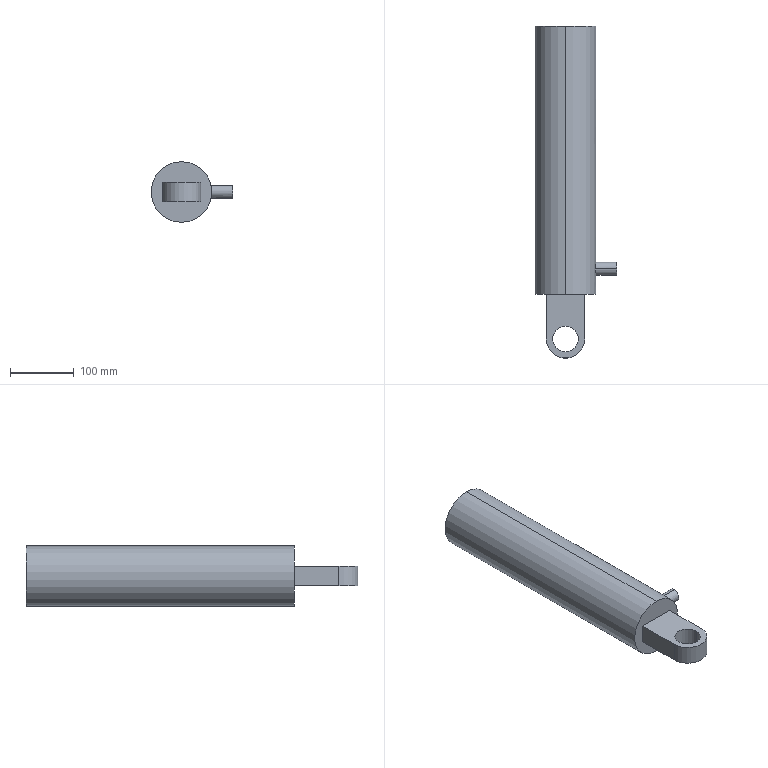Part | STEP file | Hydraulic cylinder body SLDPRT | 1 solid | 20 faces | box 127.5 x 520 x 95 mm | volume 2648079 mm3 | cylinder 12 | plane 8 | commonest cylinder face diameters 40 x4 95 x3 14 x2 20 x2 60 x1
STEP:
#1=CARTESIAN_POINT('',(80.,110.,22.));
#2=VERTEX_POINT('',#1);
#3=CARTESIAN_POINT('',(80.,110.,8.));
#4=VERTEX_POINT('',#3);
#5=CARTESIAN_POINT('',(80.,110.,15.));
#6=DIRECTION('',(1.,0.,0.));
#7=DIRECTION('',(0.,0.,-1.));
#8=AXIS2_PLACEMENT_3D('',#5,#6,#7);
#9=CIRCLE('',#8,7.);
#10=EDGE_CURVE('',#2,#4,#9,.T.);
#11=ORIENTED_EDGE('',*,*,#10,.T.);
#12=CARTESIAN_POINT('',(46.981,110.,8.));
#13=VERTEX_POINT('',#12);
#14=CARTESIAN_POINT('',(80.,110.,8.));
#15=DIRECTION('',(-1.,0.,0.));
#16=VECTOR('',#15,1000.);
#17=LINE('',#14,#16);
#18=EDGE_CURVE('',#4,#13,#17,.T.);
#19=ORIENTED_EDGE('',*,*,#18,.T.);
#20=CARTESIAN_POINT('',(46.981,110.,22.));
#21=VERTEX_POINT('',#20);
#22=CARTESIAN_POINT('',(46.981,110.,22.));
#23=CARTESIAN_POINT('',(46.981,109.537,22.));
#24=CARTESIAN_POINT('',(46.988,109.081,21.954));
#25=CARTESIAN_POINT('',(47.008,108.41,21.821));
#26=CARTESIAN_POINT('',(47.016,108.188,21.765));
#27=CARTESIAN_POINT('',(47.035,107.748,21.632));
#28=CARTESIAN_POINT('',(47.046,107.529,21.553));
#29=CARTESIAN_POINT('',(47.082,106.893,21.29));
#30=CARTESIAN_POINT('',(47.111,106.492,21.075));
#31=CARTESIAN_POINT('',(47.173,105.731,20.567));
#32=CARTESIAN_POINT('',(47.208,105.372,20.271));
#33=CARTESIAN_POINT('',(47.275,104.727,19.626));
#34=CARTESIAN_POINT('',(47.309,104.437,19.274));
#35=CARTESIAN_POINT('',(47.356,104.054,18.7));
#36=CARTESIAN_POINT('',(47.371,103.935,18.502));
#37=CARTESIAN_POINT('',(47.399,103.719,18.098));
#38=CARTESIAN_POINT('',(47.425,103.524,17.686));
#39=CARTESIAN_POINT('',(47.447,103.37,17.256));
#40=CARTESIAN_POINT('',(47.466,103.236,16.817));
#41=CARTESIAN_POINT('',(47.474,103.18,16.593));
#42=CARTESIAN_POINT('',(47.493,103.045,15.915));
#43=CARTESIAN_POINT('',(47.5,103.,15.46));
#44=CARTESIAN_POINT('',(47.5,103.,14.545));
#45=CARTESIAN_POINT('',(47.493,103.046,14.081));
#46=CARTESIAN_POINT('',(47.467,103.225,13.183));
#47=CARTESIAN_POINT('',(47.448,103.357,12.746));
#48=CARTESIAN_POINT('',(47.412,103.62,12.11));
#49=CARTESIAN_POINT('',(47.399,103.72,11.9));
#50=CARTESIAN_POINT('',(47.371,103.936,11.495));
#51=CARTESIAN_POINT('',(47.356,104.054,11.299));
#52=CARTESIAN_POINT('',(47.309,104.434,10.731));
#53=CARTESIAN_POINT('',(47.276,104.724,10.377));
#54=CARTESIAN_POINT('',(47.207,105.376,9.724));
#55=CARTESIAN_POINT('',(47.174,105.729,9.435));
#56=CARTESIAN_POINT('',(47.127,106.297,9.055));
#57=CARTESIAN_POINT('',(47.112,106.493,8.937));
#58=CARTESIAN_POINT('',(47.083,106.899,8.72));
#59=CARTESIAN_POINT('',(47.07,107.108,8.621));
#60=CARTESIAN_POINT('',(47.034,107.744,8.358));
#61=CARTESIAN_POINT('',(47.014,108.18,8.225));
#62=CARTESIAN_POINT('',(46.988,109.078,8.046));
#63=CARTESIAN_POINT('',(46.981,109.543,8.));
#64=CARTESIAN_POINT('',(46.981,110.,8.));
#65=B_SPLINE_CURVE_WITH_KNOTS('',3,(#22,#23,#24,#25,#26,#27,#28,#29,#30,#31,#32,#33,#34,#35,#36,#37,#38,#39,#40,#41,#42,#43,#44,#45,#46,#47,#48,#49,#50,#51,#52,#53,#54,#55,#56,#57,#58,#59,#60,#61,#62,#63,#64),.UNSPECIFIED.,.F.,.F.,(4,2,2,2,2,2,2,2,1,2,2,2,2,2,2,2,2,2,2,2,2,4),(0.,0.00137,0.002055,0.002739,0.004109,0.005479,0.006848,0.007533,0.008218,0.008903,0.009588,0.01096,0.01233,0.0137,0.01438,0.01507,0.01644,0.01781,0.01849,0.01918,0.02055,0.02192),.UNSPECIFIED.);
#66=EDGE_CURVE('',#21,#13,#65,.T.);
#67=ORIENTED_EDGE('',*,*,#66,.F.);
#68=CARTESIAN_POINT('',(80.,110.,22.));
#69=DIRECTION('',(-1.,0.,0.));
#70=VECTOR('',#69,1000.);
#71=LINE('',#68,#70);
#72=EDGE_CURVE('',#2,#21,#71,.T.);
#73=ORIENTED_EDGE('',*,*,#72,.F.);
#74=EDGE_LOOP('',(#11,#19,#67,#73));
#75=FACE_OUTER_BOUND('',#74,.T.);
#76=CARTESIAN_POINT('',(80.,110.,15.));
#77=DIRECTION('',(-1.,0.,0.));
#78=DIRECTION('',(0.,0.,1.));
#79=AXIS2_PLACEMENT_3D('',#76,#77,#78);
#80=CYLINDRICAL_SURFACE('',#79,7.);
#81=ADVANCED_FACE('',(#75),#80,.F.);
#82=CARTESIAN_POINT('',(80.,110.,5.));
#83=VERTEX_POINT('',#82);
#84=CARTESIAN_POINT('',(80.,110.,25.));
#85=VERTEX_POINT('',#84);
#86=CARTESIAN_POINT('',(80.,110.,15.));
#87=DIRECTION('',(1.,0.,0.));
#88=DIRECTION('',(0.,0.,-1.));
#89=AXIS2_PLACEMENT_3D('',#86,#87,#88);
#90=CIRCLE('',#89,10.);
#91=EDGE_CURVE('',#83,#85,#90,.T.);
#92=ORIENTED_EDGE('',*,*,#91,.F.);
#93=CARTESIAN_POINT('',(46.435,110.,5.));
#94=VERTEX_POINT('',#93);
#95=CARTESIAN_POINT('',(80.,110.,5.));
#96=DIRECTION('',(-1.,0.,0.));
#97=VECTOR('',#96,1000.);
#98=LINE('',#95,#97);
#99=EDGE_CURVE('',#83,#94,#98,.T.);
#100=ORIENTED_EDGE('',*,*,#99,.T.);
#101=CARTESIAN_POINT('',(46.435,110.,25.));
#102=VERTEX_POINT('',#101);
#103=CARTESIAN_POINT('',(46.435,110.,5.));
#104=CARTESIAN_POINT('',(46.435,110.653,5.));
#105=CARTESIAN_POINT('',(46.449,111.304,5.063));
#106=CARTESIAN_POINT('',(46.504,112.6,5.321));
#107=CARTESIAN_POINT('',(46.544,113.228,5.513));
#108=CARTESIAN_POINT('',(46.618,114.131,5.887));
#109=CARTESIAN_POINT('',(46.645,114.426,6.027));
#110=CARTESIAN_POINT('',(46.703,115.004,6.336));
#111=CARTESIAN_POINT('',(46.735,115.288,6.506));
#112=CARTESIAN_POINT('',(46.832,116.104,7.052));
#113=CARTESIAN_POINT('',(46.901,116.606,7.464));
#114=CARTESIAN_POINT('',(47.005,117.298,8.155));
#115=CARTESIAN_POINT('',(47.04,117.519,8.399));
#116=CARTESIAN_POINT('',(47.108,117.936,8.906));
#117=CARTESIAN_POINT('',(47.142,118.13,9.169));
#118=CARTESIAN_POINT('',(47.237,118.673,9.98));
#119=CARTESIAN_POINT('',(47.295,118.981,10.554));
#120=CARTESIAN_POINT('',(47.369,119.36,11.464));
#121=CARTESIAN_POINT('',(47.391,119.472,11.776));
#122=CARTESIAN_POINT('',(47.43,119.662,12.403));
#123=CARTESIAN_POINT('',(47.463,119.821,13.036));
#124=CARTESIAN_POINT('',(47.483,119.918,13.682));
#125=CARTESIAN_POINT('',(47.496,119.983,14.334));
#126=CARTESIAN_POINT('',(47.5,120.,14.665));
#127=CARTESIAN_POINT('',(47.5,120.,15.655));
#128=CARTESIAN_POINT('',(47.486,119.936,16.306));
#129=CARTESIAN_POINT('',(47.447,119.745,17.267));
#130=CARTESIAN_POINT('',(47.431,119.666,17.586));
#131=CARTESIAN_POINT('',(47.392,119.474,18.217));
#132=CARTESIAN_POINT('',(47.37,119.363,18.528));
#133=CARTESIAN_POINT('',(47.297,118.987,19.433));
#134=CARTESIAN_POINT('',(47.238,118.681,20.008));
#135=CARTESIAN_POINT('',(47.142,118.135,20.824));
#136=CARTESIAN_POINT('',(47.109,117.938,21.09));
#137=CARTESIAN_POINT('',(47.041,117.523,21.596));
#138=CARTESIAN_POINT('',(47.006,117.305,21.837));
#139=CARTESIAN_POINT('',(46.902,116.616,22.527));
#140=CARTESIAN_POINT('',(46.833,116.112,22.942));
#141=CARTESIAN_POINT('',(46.703,115.018,23.675));
#142=CARTESIAN_POINT('',(46.644,114.444,23.982));
#143=CARTESIAN_POINT('',(46.569,113.542,24.357));
#144=CARTESIAN_POINT('',(46.547,113.235,24.468));
#145=CARTESIAN_POINT('',(46.507,112.606,24.66));
#146=CARTESIAN_POINT('',(46.49,112.284,24.741));
#147=CARTESIAN_POINT('',(46.45,111.316,24.935));
#148=CARTESIAN_POINT('',(46.435,110.663,25.));
#149=CARTESIAN_POINT('',(46.435,110.,25.));
#150=B_SPLINE_CURVE_WITH_KNOTS('',3,(#103,#104,#105,#106,#107,#108,#109,#110,#111,#112,#113,#114,#115,#116,#117,#118,#119,#120,#121,#122,#123,#124,#125,#126,#127,#128,#129,#130,#131,#132,#133,#134,#135,#136,#137,#138,#139,#140,#141,#142,#143,#144,#145,#146,#147,#148,#149),.UNSPECIFIED.,.F.,.F.,(4,2,2,2,2,2,2,2,2,2,1,2,2,2,2,2,2,2,2,2,2,2,2,4),(0.03135,0.03331,0.03527,0.03625,0.03723,0.03919,0.04017,0.04115,0.04311,0.04409,0.04507,0.04604,0.04702,0.04898,0.04996,0.05094,0.0529,0.05388,0.05486,0.05682,0.05878,0.05976,0.06074,0.0627),.UNSPECIFIED.);
#151=EDGE_CURVE('',#94,#102,#150,.T.);
#152=ORIENTED_EDGE('',*,*,#151,.T.);
#153=CARTESIAN_POINT('',(80.,110.,25.));
#154=DIRECTION('',(-1.,0.,0.));
#155=VECTOR('',#154,1000.);
#156=LINE('',#153,#155);
#157=EDGE_CURVE('',#85,#102,#156,.T.);
#158=ORIENTED_EDGE('',*,*,#157,.F.);
#159=EDGE_LOOP('',(#92,#100,#152,#158));
#160=FACE_OUTER_BOUND('',#159,.T.);
#161=CARTESIAN_POINT('',(80.,110.,15.));
#162=DIRECTION('',(-1.,0.,0.));
#163=DIRECTION('',(0.,0.,1.));
#164=AXIS2_PLACEMENT_3D('',#161,#162,#163);
#165=CYLINDRICAL_SURFACE('',#164,10.);
#166=ADVANCED_FACE('',(#160),#165,.T.);
#167=CARTESIAN_POINT('',(0.,120.,35.));
#168=VERTEX_POINT('',#167);
#169=CARTESIAN_POINT('',(0.,120.,-5.));
#170=VERTEX_POINT('',#169);
#171=CARTESIAN_POINT('',(0.,120.,15.));
#172=DIRECTION('',(0.,-1.,0.));
#173=DIRECTION('',(0.,0.,1.));
#174=AXIS2_PLACEMENT_3D('',#171,#172,#173);
#175=CIRCLE('',#174,20.);
#176=EDGE_CURVE('',#168,#170,#175,.T.);
#177=ORIENTED_EDGE('',*,*,#176,.T.);
#178=CARTESIAN_POINT('',(0.,490.,-5.));
#179=VERTEX_POINT('',#178);
#180=CARTESIAN_POINT('',(0.,13.431,-5.));
#181=DIRECTION('',(0.,1.,0.));
#182=VECTOR('',#181,1000.);
#183=LINE('',#180,#182);
#184=EDGE_CURVE('',#170,#179,#183,.T.);
#185=ORIENTED_EDGE('',*,*,#184,.T.);
#186=CARTESIAN_POINT('',(0.,490.,35.));
#187=VERTEX_POINT('',#186);
#188=CARTESIAN_POINT('',(0.,490.,15.));
#189=DIRECTION('',(0.,1.,0.));
#190=DIRECTION('',(0.,0.,1.));
#191=AXIS2_PLACEMENT_3D('',#188,#189,#190);
#192=CIRCLE('',#191,20.);
#193=EDGE_CURVE('',#179,#187,#192,.T.);
#194=ORIENTED_EDGE('',*,*,#193,.T.);
#195=CARTESIAN_POINT('',(0.,13.431,35.));
#196=DIRECTION('',(0.,1.,0.));
#197=VECTOR('',#196,1000.);
#198=LINE('',#195,#197);
#199=EDGE_CURVE('',#168,#187,#198,.T.);
#200=ORIENTED_EDGE('',*,*,#199,.F.);
#201=EDGE_LOOP('',(#177,#185,#194,#200));
#202=FACE_OUTER_BOUND('',#201,.T.);
#203=CARTESIAN_POINT('',(0.,13.431,15.));
#204=DIRECTION('',(0.,1.,0.));
#205=DIRECTION('',(0.,0.,1.));
#206=AXIS2_PLACEMENT_3D('',#203,#204,#205);
#207=CYLINDRICAL_SURFACE('',#206,20.);
#208=ADVANCED_FACE('',(#202),#207,.F.);
#209=CARTESIAN_POINT('',(-20.,0.,30.));
#210=VERTEX_POINT('',#209);
#211=CARTESIAN_POINT('',(20.,0.,30.));
#212=VERTEX_POINT('',#211);
#213=CARTESIAN_POINT('',(0.,0.,30.));
#214=DIRECTION('',(0.,0.,1.));
#215=DIRECTION('',(1.,0.,0.));
#216=AXIS2_PLACEMENT_3D('',#213,#214,#215);
#217=CIRCLE('',#216,20.);
#218=EDGE_CURVE('',#210,#212,#217,.T.);
#219=ORIENTED_EDGE('',*,*,#218,.T.);
#220=CARTESIAN_POINT('',(20.,0.,0.));
#221=VERTEX_POINT('',#220);
#222=CARTESIAN_POINT('',(20.,0.,30.));
#223=DIRECTION('',(0.,0.,-1.));
#224=VECTOR('',#223,1000.);
#225=LINE('',#222,#224);
#226=EDGE_CURVE('',#212,#221,#225,.T.);
#227=ORIENTED_EDGE('',*,*,#226,.T.);
#228=CARTESIAN_POINT('',(-20.,0.,0.));
#229=VERTEX_POINT('',#228);
#230=CARTESIAN_POINT('',(0.,0.,0.));
#231=DIRECTION('',(0.,0.,1.));
#232=DIRECTION('',(1.,0.,0.));
#233=AXIS2_PLACEMENT_3D('',#230,#231,#232);
#234=CIRCLE('',#233,20.);
#235=EDGE_CURVE('',#229,#221,#234,.T.);
#236=ORIENTED_EDGE('',*,*,#235,.F.);
#237=CARTESIAN_POINT('',(-20.,0.,30.));
#238=DIRECTION('',(0.,0.,-1.));
#239=VECTOR('',#238,1000.);
#240=LINE('',#237,#239);
#241=EDGE_CURVE('',#210,#229,#240,.T.);
#242=ORIENTED_EDGE('',*,*,#241,.F.);
#243=EDGE_LOOP('',(#219,#227,#236,#242));
#244=FACE_OUTER_BOUND('',#243,.T.);
#245=CARTESIAN_POINT('',(0.,0.,30.));
#246=DIRECTION('',(0.,0.,-1.));
#247=DIRECTION('',(-1.,0.,0.));
#248=AXIS2_PLACEMENT_3D('',#245,#246,#247);
#249=CYLINDRICAL_SURFACE('',#248,20.);
#250=ADVANCED_FACE('',(#244),#249,.F.);
#251=CARTESIAN_POINT('',(46.435,110.,25.));
#252=CARTESIAN_POINT('',(46.435,109.337,25.));
#253=CARTESIAN_POINT('',(46.45,108.686,24.935));
#254=CARTESIAN_POINT('',(46.49,107.725,24.743));
#255=CARTESIAN_POINT('',(46.507,107.408,24.664));
#256=CARTESIAN_POINT('',(46.546,106.779,24.473));
#257=CARTESIAN_POINT('',(46.569,106.467,24.361));
#258=CARTESIAN_POINT('',(46.643,105.559,23.984));
#259=CARTESIAN_POINT('',(46.702,104.985,23.676));
#260=CARTESIAN_POINT('',(46.799,104.171,23.132));
#261=CARTESIAN_POINT('',(46.833,103.906,22.936));
#262=CARTESIAN_POINT('',(46.902,103.399,22.519));
#263=CARTESIAN_POINT('',(46.936,103.157,22.299));
#264=CARTESIAN_POINT('',(47.04,102.468,21.61));
#265=CARTESIAN_POINT('',(47.109,102.054,21.107));
#266=CARTESIAN_POINT('',(47.206,101.506,20.288));
#267=CARTESIAN_POINT('',(47.236,101.336,20.005));
#268=CARTESIAN_POINT('',(47.294,101.028,19.429));
#269=CARTESIAN_POINT('',(47.321,100.889,19.135));
#270=CARTESIAN_POINT('',(47.369,100.639,18.533));
#271=CARTESIAN_POINT('',(47.391,100.529,18.226));
#272=CARTESIAN_POINT('',(47.43,100.338,17.599));
#273=CARTESIAN_POINT('',(47.446,100.257,17.277));
#274=CARTESIAN_POINT('',(47.486,100.064,16.308));
#275=CARTESIAN_POINT('',(47.5,100.,15.658));
#276=CARTESIAN_POINT('',(47.5,100.,14.35));
#277=CARTESIAN_POINT('',(47.486,100.065,13.685));
#278=CARTESIAN_POINT('',(47.433,100.322,12.401));
#279=CARTESIAN_POINT('',(47.394,100.511,11.776));
#280=CARTESIAN_POINT('',(47.321,100.888,10.867));
#281=CARTESIAN_POINT('',(47.294,101.03,10.567));
#282=CARTESIAN_POINT('',(47.236,101.339,9.99));
#283=CARTESIAN_POINT('',(47.205,101.507,9.71));
#284=CARTESIAN_POINT('',(47.142,101.869,9.17));
#285=CARTESIAN_POINT('',(47.108,102.063,8.908));
#286=CARTESIAN_POINT('',(47.041,102.477,8.404));
#287=CARTESIAN_POINT('',(47.006,102.698,8.16));
#288=CARTESIAN_POINT('',(46.901,103.395,7.463));
#289=CARTESIAN_POINT('',(46.832,103.898,7.051));
#290=CARTESIAN_POINT('',(46.735,104.709,6.508));
#291=CARTESIAN_POINT('',(46.704,104.989,6.34));
#292=CARTESIAN_POINT('',(46.646,105.568,6.03));
#293=CARTESIAN_POINT('',(46.618,105.867,5.888));
#294=CARTESIAN_POINT('',(46.544,106.773,5.512));
#295=CARTESIAN_POINT('',(46.504,107.397,5.323));
#296=CARTESIAN_POINT('',(46.463,108.361,5.13));
#297=CARTESIAN_POINT('',(46.453,108.689,5.081));
#298=CARTESIAN_POINT('',(46.439,109.346,5.016));
#299=CARTESIAN_POINT('',(46.435,109.673,5.));
#300=CARTESIAN_POINT('',(46.435,110.,5.));
#301=B_SPLINE_CURVE_WITH_KNOTS('',3,(#251,#252,#253,#254,#255,#256,#257,#258,#259,#260,#261,#262,#263,#264,#265,#266,#267,#268,#269,#270,#271,#272,#273,#274,#275,#276,#277,#278,#279,#280,#281,#282,#283,#284,#285,#286,#287,#288,#289,#290,#291,#292,#293,#294,#295,#296,#297,#298,#299,#300),.UNSPECIFIED.,.F.,.F.,(4,2,2,2,2,2,2,2,2,2,2,2,2,2,2,2,2,2,2,2,2,2,2,2,4),(0.,0.00196,0.002939,0.003919,0.005879,0.006858,0.007838,0.009798,0.01078,0.01176,0.01274,0.01372,0.01568,0.01764,0.0196,0.02057,0.02155,0.02253,0.02351,0.02547,0.02645,0.02743,0.02939,0.03037,0.03135),.UNSPECIFIED.);
#302=EDGE_CURVE('',#102,#94,#301,.T.);
#303=ORIENTED_EDGE('',*,*,#302,.F.);
#304=ORIENTED_EDGE('',*,*,#151,.F.);
#305=EDGE_LOOP('',(#303,#304));
#306=FACE_BOUND('',#305,.T.);
#307=CARTESIAN_POINT('',(0.,490.,62.5));
#308=VERTEX_POINT('',#307);
#309=CARTESIAN_POINT('',(0.,490.,-32.5));
#310=VERTEX_POINT('',#309);
#311=CARTESIAN_POINT('',(0.,490.,15.));
#312=DIRECTION('',(0.,1.,0.));
#313=DIRECTION('',(0.,0.,1.));
#314=AXIS2_PLACEMENT_3D('',#311,#312,#313);
#315=CIRCLE('',#314,47.5);
#316=EDGE_CURVE('',#308,#310,#315,.T.);
#317=ORIENTED_EDGE('',*,*,#316,.F.);
#318=CARTESIAN_POINT('',(0.,70.,62.5));
#319=VERTEX_POINT('',#318);
#320=CARTESIAN_POINT('',(0.,490.,62.5));
#321=DIRECTION('',(0.,-1.,0.));
#322=VECTOR('',#321,1000.);
#323=LINE('',#320,#322);
#324=EDGE_CURVE('',#308,#319,#323,.T.);
#325=ORIENTED_EDGE('',*,*,#324,.T.);
#326=CARTESIAN_POINT('',(0.,70.,-32.5));
#327=VERTEX_POINT('',#326);
#328=CARTESIAN_POINT('',(0.,70.,15.));
#329=DIRECTION('',(0.,1.,0.));
#330=DIRECTION('',(0.,0.,1.));
#331=AXIS2_PLACEMENT_3D('',#328,#329,#330);
#332=CIRCLE('',#331,47.5);
#333=EDGE_CURVE('',#319,#327,#332,.T.);
#334=ORIENTED_EDGE('',*,*,#333,.T.);
#335=CARTESIAN_POINT('',(0.,490.,-32.5));
#336=DIRECTION('',(0.,-1.,0.));
#337=VECTOR('',#336,1000.);
#338=LINE('',#335,#337);
#339=EDGE_CURVE('',#310,#327,#338,.T.);
#340=ORIENTED_EDGE('',*,*,#339,.F.);
#341=EDGE_LOOP('',(#317,#325,#334,#340));
#342=FACE_OUTER_BOUND('',#341,.T.);
#343=CARTESIAN_POINT('',(0.,490.,15.));
#344=DIRECTION('',(0.,-1.,0.));
#345=DIRECTION('',(0.,0.,-1.));
#346=AXIS2_PLACEMENT_3D('',#343,#344,#345);
#347=CYLINDRICAL_SURFACE('',#346,47.5);
#348=ADVANCED_FACE('',(#306,#342),#347,.T.);
#349=ORIENTED_EDGE('',*,*,#324,.F.);
#350=CARTESIAN_POINT('',(0.,490.,15.));
#351=DIRECTION('',(0.,1.,0.));
#352=DIRECTION('',(0.,0.,1.));
#353=AXIS2_PLACEMENT_3D('',#350,#351,#352);
#354=CIRCLE('',#353,47.5);
#355=EDGE_CURVE('',#310,#308,#354,.T.);
#356=ORIENTED_EDGE('',*,*,#355,.F.);
#357=ORIENTED_EDGE('',*,*,#339,.T.);
#358=CARTESIAN_POINT('',(0.,70.,15.));
#359=DIRECTION('',(0.,1.,0.));
#360=DIRECTION('',(0.,0.,1.));
#361=AXIS2_PLACEMENT_3D('',#358,#359,#360);
#362=CIRCLE('',#361,47.5);
#363=EDGE_CURVE('',#327,#319,#362,.T.);
#364=ORIENTED_EDGE('',*,*,#363,.T.);
#365=EDGE_LOOP('',(#349,#356,#357,#364));
#366=FACE_OUTER_BOUND('',#365,.T.);
#367=CARTESIAN_POINT('',(0.,490.,15.));
#368=DIRECTION('',(0.,-1.,0.));
#369=DIRECTION('',(0.,0.,-1.));
#370=AXIS2_PLACEMENT_3D('',#367,#368,#369);
#371=CYLINDRICAL_SURFACE('',#370,47.5);
#372=ADVANCED_FACE('',(#366),#371,.T.);
#373=CARTESIAN_POINT('',(-30.,0.,30.));
#374=VERTEX_POINT('',#373);
#375=CARTESIAN_POINT('',(30.,0.,30.));
#376=VERTEX_POINT('',#375);
#377=CARTESIAN_POINT('',(0.,0.,30.));
#378=DIRECTION('',(0.,0.,1.));
#379=DIRECTION('',(1.,0.,0.));
#380=AXIS2_PLACEMENT_3D('',#377,#378,#379);
#381=CIRCLE('',#380,30.);
#382=EDGE_CURVE('',#374,#376,#381,.T.);
#383=ORIENTED_EDGE('',*,*,#382,.T.);
#384=CARTESIAN_POINT('',(30.,70.,30.));
#385=VERTEX_POINT('',#384);
#386=CARTESIAN_POINT('',(30.,70.,30.));
#387=DIRECTION('',(0.,1.,0.));
#388=VECTOR('',#387,1000.);
#389=LINE('',#386,#388);
#390=EDGE_CURVE('',#376,#385,#389,.T.);
#391=ORIENTED_EDGE('',*,*,#390,.T.);
#392=CARTESIAN_POINT('',(-30.,70.,30.));
#393=VERTEX_POINT('',#392);
#394=CARTESIAN_POINT('',(-30.,70.,30.));
#395=DIRECTION('',(-1.,0.,0.));
#396=VECTOR('',#395,1000.);
#397=LINE('',#394,#396);
#398=EDGE_CURVE('',#385,#393,#397,.T.);
#399=ORIENTED_EDGE('',*,*,#398,.T.);
#400=CARTESIAN_POINT('',(-30.,0.,30.));
#401=DIRECTION('',(0.,-1.,0.));
#402=VECTOR('',#401,1000.);
#403=LINE('',#400,#402);
#404=EDGE_CURVE('',#393,#374,#403,.T.);
#405=ORIENTED_EDGE('',*,*,#404,.T.);
#406=EDGE_LOOP('',(#383,#391,#399,#405));
#407=FACE_OUTER_BOUND('',#406,.T.);
#408=ORIENTED_EDGE('',*,*,#218,.F.);
#409=CARTESIAN_POINT('',(0.,0.,30.));
#410=DIRECTION('',(0.,0.,1.));
#411=DIRECTION('',(1.,0.,0.));
#412=AXIS2_PLACEMENT_3D('',#409,#410,#411);
#413=CIRCLE('',#412,20.);
#414=EDGE_CURVE('',#212,#210,#413,.T.);
#415=ORIENTED_EDGE('',*,*,#414,.F.);
#416=EDGE_LOOP('',(#408,#415));
#417=FACE_BOUND('',#416,.T.);
#418=CARTESIAN_POINT('',(0.,0.,30.));
#419=DIRECTION('',(0.,0.,1.));
#420=DIRECTION('',(1.,0.,0.));
#421=AXIS2_PLACEMENT_3D('',#418,#419,#420);
#422=PLANE('',#421);
#423=ADVANCED_FACE('',(#407,#417),#422,.T.);
#424=CARTESIAN_POINT('',(-30.,0.,0.));
#425=VERTEX_POINT('',#424);
#426=CARTESIAN_POINT('',(30.,0.,0.));
#427=VERTEX_POINT('',#426);
#428=CARTESIAN_POINT('',(0.,0.,0.));
#429=DIRECTION('',(0.,0.,1.));
#430=DIRECTION('',(1.,0.,0.));
#431=AXIS2_PLACEMENT_3D('',#428,#429,#430);
#432=CIRCLE('',#431,30.);
#433=EDGE_CURVE('',#425,#427,#432,.T.);
#434=ORIENTED_EDGE('',*,*,#433,.F.);
#435=CARTESIAN_POINT('',(-30.,70.,0.));
#436=VERTEX_POINT('',#435);
#437=CARTESIAN_POINT('',(-30.,0.,0.));
#438=DIRECTION('',(0.,-1.,0.));
#439=VECTOR('',#438,1000.);
#440=LINE('',#437,#439);
#441=EDGE_CURVE('',#436,#425,#440,.T.);
#442=ORIENTED_EDGE('',*,*,#441,.F.);
#443=CARTESIAN_POINT('',(30.,70.,0.));
#444=VERTEX_POINT('',#443);
#445=CARTESIAN_POINT('',(-30.,70.,0.));
#446=DIRECTION('',(-1.,0.,0.));
#447=VECTOR('',#446,1000.);
#448=LINE('',#445,#447);
#449=EDGE_CURVE('',#444,#436,#448,.T.);
#450=ORIENTED_EDGE('',*,*,#449,.F.);
#451=CARTESIAN_POINT('',(30.,70.,0.));
#452=DIRECTION('',(0.,1.,0.));
#453=VECTOR('',#452,1000.);
#454=LINE('',#451,#453);
#455=EDGE_CURVE('',#427,#444,#454,.T.);
#456=ORIENTED_EDGE('',*,*,#455,.F.);
#457=EDGE_LOOP('',(#434,#442,#450,#456));
#458=FACE_OUTER_BOUND('',#457,.T.);
#459=ORIENTED_EDGE('',*,*,#235,.T.);
#460=CARTESIAN_POINT('',(0.,0.,0.));
#461=DIRECTION('',(0.,0.,1.));
#462=DIRECTION('',(1.,0.,0.));
#463=AXIS2_PLACEMENT_3D('',#460,#461,#462);
#464=CIRCLE('',#463,20.);
#465=EDGE_CURVE('',#221,#229,#464,.T.);
#466=ORIENTED_EDGE('',*,*,#465,.T.);
#467=EDGE_LOOP('',(#459,#466));
#468=FACE_BOUND('',#467,.T.);
#469=CARTESIAN_POINT('',(0.,0.,0.));
#470=DIRECTION('',(0.,0.,1.));
#471=DIRECTION('',(1.,0.,0.));
#472=AXIS2_PLACEMENT_3D('',#469,#470,#471);
#473=PLANE('',#472);
#474=ADVANCED_FACE('',(#458,#468),#473,.F.);
#475=ORIENTED_EDGE('',*,*,#433,.T.);
#476=CARTESIAN_POINT('',(30.,0.,30.));
#477=DIRECTION('',(0.,0.,-1.));
#478=VECTOR('',#477,1000.);
#479=LINE('',#476,#478);
#480=EDGE_CURVE('',#376,#427,#479,.T.);
#481=ORIENTED_EDGE('',*,*,#480,.F.);
#482=ORIENTED_EDGE('',*,*,#382,.F.);
#483=CARTESIAN_POINT('',(-30.,0.,30.));
#484=DIRECTION('',(0.,0.,-1.));
#485=VECTOR('',#484,1000.);
#486=LINE('',#483,#485);
#487=EDGE_CURVE('',#374,#425,#486,.T.);
#488=ORIENTED_EDGE('',*,*,#487,.T.);
#489=EDGE_LOOP('',(#475,#481,#482,#488));
#490=FACE_OUTER_BOUND('',#489,.T.);
#491=CARTESIAN_POINT('',(0.,0.,30.));
#492=DIRECTION('',(0.,0.,-1.));
#493=DIRECTION('',(-1.,0.,0.));
#494=AXIS2_PLACEMENT_3D('',#491,#492,#493);
#495=CYLINDRICAL_SURFACE('',#494,30.);
#496=ADVANCED_FACE('',(#490),#495,.T.);
#497=ORIENTED_EDGE('',*,*,#455,.T.);
#498=CARTESIAN_POINT('',(30.,70.,30.));
#499=DIRECTION('',(0.,0.,-1.));
#500=VECTOR('',#499,1000.);
#501=LINE('',#498,#500);
#502=EDGE_CURVE('',#385,#444,#501,.T.);
#503=ORIENTED_EDGE('',*,*,#502,.F.);
#504=ORIENTED_EDGE('',*,*,#390,.F.);
#505=ORIENTED_EDGE('',*,*,#480,.T.);
#506=EDGE_LOOP('',(#497,#503,#504,#505));
#507=FACE_OUTER_BOUND('',#506,.T.);
#508=CARTESIAN_POINT('',(30.,70.,30.));
#509=DIRECTION('',(-1.,0.,0.));
#510=DIRECTION('',(0.,0.,1.));
#511=AXIS2_PLACEMENT_3D('',#508,#509,#510);
#512=PLANE('',#511);
#513=ADVANCED_FACE('',(#507),#512,.F.);
#514=ORIENTED_EDGE('',*,*,#441,.T.);
#515=ORIENTED_EDGE('',*,*,#487,.F.);
#516=ORIENTED_EDGE('',*,*,#404,.F.);
#517=CARTESIAN_POINT('',(-30.,70.,30.));
#518=DIRECTION('',(0.,0.,-1.));
#519=VECTOR('',#518,1000.);
#520=LINE('',#517,#519);
#521=EDGE_CURVE('',#393,#436,#520,.T.);
#522=ORIENTED_EDGE('',*,*,#521,.T.);
#523=EDGE_LOOP('',(#514,#515,#516,#522));
#524=FACE_OUTER_BOUND('',#523,.T.);
#525=CARTESIAN_POINT('',(-30.,0.,30.));
#526=DIRECTION('',(1.,0.,0.));
#527=DIRECTION('',(0.,0.,-1.));
#528=AXIS2_PLACEMENT_3D('',#525,#526,#527);
#529=PLANE('',#528);
#530=ADVANCED_FACE('',(#524),#529,.F.);
#531=ORIENTED_EDGE('',*,*,#226,.F.);
#532=ORIENTED_EDGE('',*,*,#414,.T.);
#533=ORIENTED_EDGE('',*,*,#241,.T.);
#534=ORIENTED_EDGE('',*,*,#465,.F.);
#535=EDGE_LOOP('',(#531,#532,#533,#534));
#536=FACE_OUTER_BOUND('',#535,.T.);
#537=CARTESIAN_POINT('',(0.,0.,30.));
#538=DIRECTION('',(0.,0.,-1.));
#539=DIRECTION('',(-1.,0.,0.));
#540=AXIS2_PLACEMENT_3D('',#537,#538,#539);
#541=CYLINDRICAL_SURFACE('',#540,20.);
#542=ADVANCED_FACE('',(#536),#541,.F.);
#543=ORIENTED_EDGE('',*,*,#363,.F.);
#544=ORIENTED_EDGE('',*,*,#333,.F.);
#545=EDGE_LOOP('',(#543,#544));
#546=FACE_OUTER_BOUND('',#545,.T.);
#547=ORIENTED_EDGE('',*,*,#502,.T.);
#548=ORIENTED_EDGE('',*,*,#449,.T.);
#549=ORIENTED_EDGE('',*,*,#521,.F.);
#550=ORIENTED_EDGE('',*,*,#398,.F.);
#551=EDGE_LOOP('',(#547,#548,#549,#550));
#552=FACE_BOUND('',#551,.T.);
#553=CARTESIAN_POINT('',(0.,70.,15.));
#554=DIRECTION('',(0.,1.,0.));
#555=DIRECTION('',(0.,0.,1.));
#556=AXIS2_PLACEMENT_3D('',#553,#554,#555);
#557=PLANE('',#556);
#558=ADVANCED_FACE('',(#546,#552),#557,.F.);
#559=CARTESIAN_POINT('',(0.,490.,15.));
#560=DIRECTION('',(0.,1.,0.));
#561=DIRECTION('',(0.,0.,1.));
#562=AXIS2_PLACEMENT_3D('',#559,#560,#561);
#563=CIRCLE('',#562,20.);
#564=EDGE_CURVE('',#187,#179,#563,.T.);
#565=ORIENTED_EDGE('',*,*,#564,.F.);
#566=ORIENTED_EDGE('',*,*,#193,.F.);
#567=EDGE_LOOP('',(#565,#566));
#568=FACE_BOUND('',#567,.T.);
#569=ORIENTED_EDGE('',*,*,#355,.T.);
#570=ORIENTED_EDGE('',*,*,#316,.T.);
#571=EDGE_LOOP('',(#569,#570));
#572=FACE_OUTER_BOUND('',#571,.T.);
#573=CARTESIAN_POINT('',(0.,490.,15.));
#574=DIRECTION('',(0.,1.,0.));
#575=DIRECTION('',(0.,0.,1.));
#576=AXIS2_PLACEMENT_3D('',#573,#574,#575);
#577=PLANE('',#576);
#578=ADVANCED_FACE('',(#568,#572),#577,.T.);
#579=ORIENTED_EDGE('',*,*,#184,.F.);
#580=CARTESIAN_POINT('',(0.,120.,15.));
#581=DIRECTION('',(0.,-1.,0.));
#582=DIRECTION('',(0.,0.,1.));
#583=AXIS2_PLACEMENT_3D('',#580,#581,#582);
#584=CIRCLE('',#583,20.);
#585=EDGE_CURVE('',#170,#168,#584,.T.);
#586=ORIENTED_EDGE('',*,*,#585,.T.);
#587=ORIENTED_EDGE('',*,*,#199,.T.);
#588=ORIENTED_EDGE('',*,*,#564,.T.);
#589=EDGE_LOOP('',(#579,#586,#587,#588));
#590=FACE_OUTER_BOUND('',#589,.T.);
#591=CARTESIAN_POINT('',(0.,13.431,15.));
#592=DIRECTION('',(0.,1.,0.));
#593=DIRECTION('',(0.,0.,1.));
#594=AXIS2_PLACEMENT_3D('',#591,#592,#593);
#595=CYLINDRICAL_SURFACE('',#594,20.);
#596=ADVANCED_FACE('',(#590),#595,.F.);
#597=ORIENTED_EDGE('',*,*,#176,.F.);
#598=ORIENTED_EDGE('',*,*,#585,.F.);
#599=EDGE_LOOP('',(#597,#598));
#600=FACE_OUTER_BOUND('',#599,.T.);
#601=CARTESIAN_POINT('',(0.,120.,15.));
#602=DIRECTION('',(0.,1.,0.));
#603=DIRECTION('',(0.,0.,1.));
#604=AXIS2_PLACEMENT_3D('',#601,#602,#603);
#605=PLANE('',#604);
#606=ADVANCED_FACE('',(#600),#605,.T.);
#607=ORIENTED_EDGE('',*,*,#99,.F.);
#608=CARTESIAN_POINT('',(80.,110.,15.));
#609=DIRECTION('',(1.,0.,0.));
#610=DIRECTION('',(0.,0.,-1.));
#611=AXIS2_PLACEMENT_3D('',#608,#609,#610);
#612=CIRCLE('',#611,10.);
#613=EDGE_CURVE('',#85,#83,#612,.T.);
#614=ORIENTED_EDGE('',*,*,#613,.F.);
#615=ORIENTED_EDGE('',*,*,#157,.T.);
#616=ORIENTED_EDGE('',*,*,#302,.T.);
#617=EDGE_LOOP('',(#607,#614,#615,#616));
#618=FACE_OUTER_BOUND('',#617,.T.);
#619=CARTESIAN_POINT('',(80.,110.,15.));
#620=DIRECTION('',(-1.,0.,0.));
#621=DIRECTION('',(0.,0.,1.));
#622=AXIS2_PLACEMENT_3D('',#619,#620,#621);
#623=CYLINDRICAL_SURFACE('',#622,10.);
#624=ADVANCED_FACE('',(#618),#623,.T.);
#625=ORIENTED_EDGE('',*,*,#18,.F.);
#626=CARTESIAN_POINT('',(80.,110.,15.));
#627=DIRECTION('',(1.,0.,0.));
#628=DIRECTION('',(0.,0.,-1.));
#629=AXIS2_PLACEMENT_3D('',#626,#627,#628);
#630=CIRCLE('',#629,7.);
#631=EDGE_CURVE('',#4,#2,#630,.T.);
#632=ORIENTED_EDGE('',*,*,#631,.T.);
#633=ORIENTED_EDGE('',*,*,#72,.T.);
#634=CARTESIAN_POINT('',(46.981,110.,8.));
#635=CARTESIAN_POINT('',(46.981,110.457,8.));
#636=CARTESIAN_POINT('',(46.988,110.912,8.044));
#637=CARTESIAN_POINT('',(47.008,111.59,8.179));
#638=CARTESIAN_POINT('',(47.016,111.815,8.235));
#639=CARTESIAN_POINT('',(47.035,112.253,8.369));
#640=CARTESIAN_POINT('',(47.057,112.683,8.523));
#641=CARTESIAN_POINT('',(47.083,113.096,8.718));
#642=CARTESIAN_POINT('',(47.111,113.5,8.933));
#643=CARTESIAN_POINT('',(47.126,113.699,9.053));
#644=CARTESIAN_POINT('',(47.174,114.272,9.435));
#645=CARTESIAN_POINT('',(47.207,114.624,9.725));
#646=CARTESIAN_POINT('',(47.275,115.269,10.369));
#647=CARTESIAN_POINT('',(47.309,115.565,10.729));
#648=CARTESIAN_POINT('',(47.372,116.073,11.488));
#649=CARTESIAN_POINT('',(47.4,116.288,11.89));
#650=CARTESIAN_POINT('',(47.436,116.552,12.526));
#651=CARTESIAN_POINT('',(47.447,116.631,12.744));
#652=CARTESIAN_POINT('',(47.466,116.764,13.184));
#653=CARTESIAN_POINT('',(47.474,116.82,13.405));
#654=CARTESIAN_POINT('',(47.493,116.954,14.077));
#655=CARTESIAN_POINT('',(47.5,117.,14.533));
#656=CARTESIAN_POINT('',(47.5,117.,15.458));
#657=CARTESIAN_POINT('',(47.493,116.955,15.913));
#658=CARTESIAN_POINT('',(47.474,116.822,16.585));
#659=CARTESIAN_POINT('',(47.466,116.767,16.807));
#660=CARTESIAN_POINT('',(47.447,116.633,17.248));
#661=CARTESIAN_POINT('',(47.436,116.555,17.466));
#662=CARTESIAN_POINT('',(47.401,116.292,18.101));
#663=CARTESIAN_POINT('',(47.372,116.078,18.503));
#664=CARTESIAN_POINT('',(47.325,115.697,19.074));
#665=CARTESIAN_POINT('',(47.309,115.559,19.26));
#666=CARTESIAN_POINT('',(47.276,115.268,19.616));
#667=CARTESIAN_POINT('',(47.259,115.114,19.785));
#668=CARTESIAN_POINT('',(47.208,114.631,20.269));
#669=CARTESIAN_POINT('',(47.174,114.279,20.559));
#670=CARTESIAN_POINT('',(47.111,113.514,21.072));
#671=CARTESIAN_POINT('',(47.082,113.109,21.288));
#672=CARTESIAN_POINT('',(47.046,112.477,21.551));
#673=CARTESIAN_POINT('',(47.035,112.263,21.628));
#674=CARTESIAN_POINT('',(47.016,111.824,21.762));
#675=CARTESIAN_POINT('',(47.008,111.599,21.819));
#676=CARTESIAN_POINT('',(46.988,110.921,21.954));
#677=CARTESIAN_POINT('',(46.981,110.463,22.));
#678=CARTESIAN_POINT('',(46.981,110.,22.));
#679=B_SPLINE_CURVE_WITH_KNOTS('',3,(#634,#635,#636,#637,#638,#639,#640,#641,#642,#643,#644,#645,#646,#647,#648,#649,#650,#651,#652,#653,#654,#655,#656,#657,#658,#659,#660,#661,#662,#663,#664,#665,#666,#667,#668,#669,#670,#671,#672,#673,#674,#675,#676,#677,#678),.UNSPECIFIED.,.F.,.F.,(4,2,2,1,2,2,2,2,2,2,2,2,2,2,2,2,2,2,2,2,2,2,4),(0.02192,0.02328,0.02397,0.02465,0.02534,0.02602,0.02739,0.02876,0.03013,0.03082,0.0315,0.03287,0.03424,0.03492,0.03561,0.03698,0.03766,0.03835,0.03972,0.04109,0.04177,0.04246,0.04382),.UNSPECIFIED.);
#680=EDGE_CURVE('',#13,#21,#679,.T.);
#681=ORIENTED_EDGE('',*,*,#680,.F.);
#682=EDGE_LOOP('',(#625,#632,#633,#681));
#683=FACE_OUTER_BOUND('',#682,.T.);
#684=CARTESIAN_POINT('',(80.,110.,15.));
#685=DIRECTION('',(-1.,0.,0.));
#686=DIRECTION('',(0.,0.,1.));
#687=AXIS2_PLACEMENT_3D('',#684,#685,#686);
#688=CYLINDRICAL_SURFACE('',#687,7.);
#689=ADVANCED_FACE('',(#683),#688,.F.);
#690=ORIENTED_EDGE('',*,*,#613,.T.);
#691=ORIENTED_EDGE('',*,*,#91,.T.);
#692=EDGE_LOOP('',(#690,#691));
#693=FACE_OUTER_BOUND('',#692,.T.);
#694=ORIENTED_EDGE('',*,*,#10,.F.);
#695=ORIENTED_EDGE('',*,*,#631,.F.);
#696=EDGE_LOOP('',(#694,#695));
#697=FACE_BOUND('',#696,.T.);
#698=CARTESIAN_POINT('',(80.,110.,15.));
#699=DIRECTION('',(1.,0.,0.));
#700=DIRECTION('',(0.,0.,-1.));
#701=AXIS2_PLACEMENT_3D('',#698,#699,#700);
#702=PLANE('',#701);
#703=ADVANCED_FACE('',(#693,#697),#702,.T.);
#704=ORIENTED_EDGE('',*,*,#66,.T.);
#705=ORIENTED_EDGE('',*,*,#680,.T.);
#706=EDGE_LOOP('',(#704,#705));
#707=FACE_OUTER_BOUND('',#706,.T.);
#708=CARTESIAN_POINT('',(0.,490.,15.));
#709=DIRECTION('',(0.,-1.,0.));
#710=DIRECTION('',(0.,0.,-1.));
#711=AXIS2_PLACEMENT_3D('',#708,#709,#710);
#712=CYLINDRICAL_SURFACE('',#711,47.5);
#713=ADVANCED_FACE('',(#707),#712,.T.);
#714=CLOSED_SHELL('',(#81,#166,#208,#250,#348,#372,#423,#474,#496,#513,#530,#542,#558,#578,#596,#606,#624,#689,#703,#713));
#715=MANIFOLD_SOLID_BREP('',#714);
#716=CARTESIAN_POINT('',(0.,0.,0.));
#717=DIRECTION('',(0.,0.,1.));
#718=DIRECTION('',(1.,0.,0.));
#719=AXIS2_PLACEMENT_3D('',#716,#717,#718);
#720=(LENGTH_UNIT()NAMED_UNIT(*)SI_UNIT(.MILLI.,.METRE.));
#721=UNCERTAINTY_MEASURE_WITH_UNIT(LENGTH_MEASURE(0.00001),#720,'','');
#722=(NAMED_UNIT(*)PLANE_ANGLE_UNIT()SI_UNIT($,.RADIAN.));
#723=(NAMED_UNIT(*)SI_UNIT($,.STERADIAN.)SOLID_ANGLE_UNIT());
#724=(GEOMETRIC_REPRESENTATION_CONTEXT(3)GLOBAL_UNCERTAINTY_ASSIGNED_CONTEXT((#721))GLOBAL_UNIT_ASSIGNED_CONTEXT((#720,#722,#723))REPRESENTATION_CONTEXT('',''));
#725=ADVANCED_BREP_SHAPE_REPRESENTATION('',(#715,#719),#724);